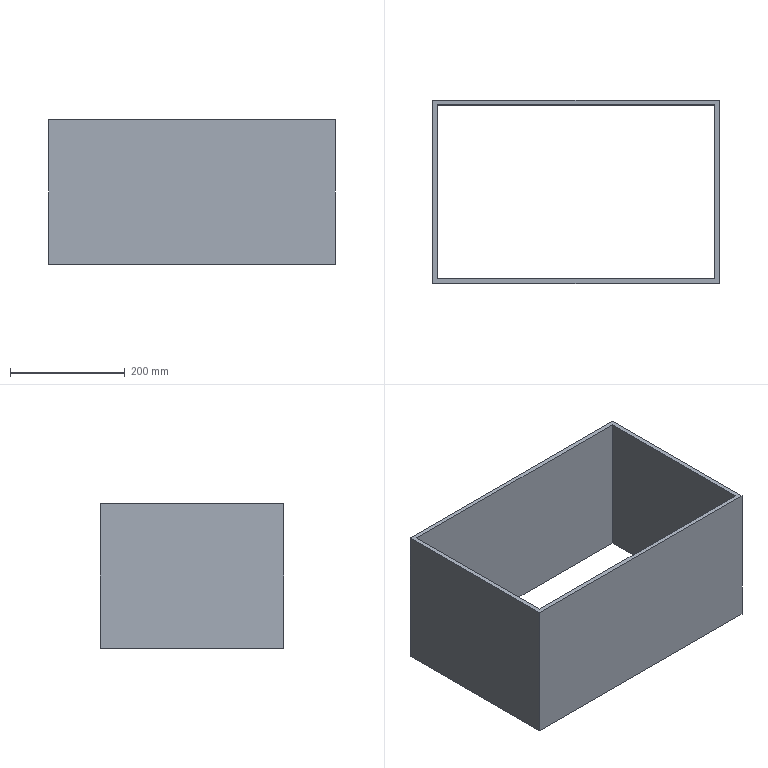Part | SolidWorks | features Extrusion 1 | 1 solid | 10 faces | box 500 x 320 x 252.7 mm | volume 3250733 mm3 | plane 10
STEP:
#1=CARTESIAN_POINT('',(0.,320.,252.7));
#2=VERTEX_POINT('',#1);
#3=CARTESIAN_POINT('',(0.,0.,252.7));
#4=VERTEX_POINT('',#3);
#5=CARTESIAN_POINT('',(0.,0.,252.7));
#6=DIRECTION('',(0.,-1.,0.));
#7=VECTOR('',#6,1000.);
#8=LINE('',#5,#7);
#9=EDGE_CURVE('',#2,#4,#8,.T.);
#10=ORIENTED_EDGE('',*,*,#9,.T.);
#11=CARTESIAN_POINT('',(500.,0.,252.7));
#12=VERTEX_POINT('',#11);
#13=CARTESIAN_POINT('',(0.,0.,252.7));
#14=DIRECTION('',(1.,0.,0.));
#15=VECTOR('',#14,1000.);
#16=LINE('',#13,#15);
#17=EDGE_CURVE('',#4,#12,#16,.T.);
#18=ORIENTED_EDGE('',*,*,#17,.T.);
#19=CARTESIAN_POINT('',(500.,320.,252.7));
#20=VERTEX_POINT('',#19);
#21=CARTESIAN_POINT('',(500.,0.,252.7));
#22=DIRECTION('',(0.,1.,0.));
#23=VECTOR('',#22,1000.);
#24=LINE('',#21,#23);
#25=EDGE_CURVE('',#12,#20,#24,.T.);
#26=ORIENTED_EDGE('',*,*,#25,.T.);
#27=CARTESIAN_POINT('',(0.,320.,252.7));
#28=DIRECTION('',(-1.,0.,0.));
#29=VECTOR('',#28,1000.);
#30=LINE('',#27,#29);
#31=EDGE_CURVE('',#20,#2,#30,.T.);
#32=ORIENTED_EDGE('',*,*,#31,.T.);
#33=EDGE_LOOP('',(#10,#18,#26,#32));
#34=FACE_OUTER_BOUND('',#33,.T.);
#35=CARTESIAN_POINT('',(8.,312.,252.7));
#36=VERTEX_POINT('',#35);
#37=CARTESIAN_POINT('',(8.,8.,252.7));
#38=VERTEX_POINT('',#37);
#39=CARTESIAN_POINT('',(8.,312.,252.7));
#40=DIRECTION('',(0.,-1.,0.));
#41=VECTOR('',#40,1000.);
#42=LINE('',#39,#41);
#43=EDGE_CURVE('',#36,#38,#42,.T.);
#44=ORIENTED_EDGE('',*,*,#43,.F.);
#45=CARTESIAN_POINT('',(492.,312.,252.7));
#46=VERTEX_POINT('',#45);
#47=CARTESIAN_POINT('',(8.,312.,252.7));
#48=DIRECTION('',(-1.,0.,0.));
#49=VECTOR('',#48,1000.);
#50=LINE('',#47,#49);
#51=EDGE_CURVE('',#46,#36,#50,.T.);
#52=ORIENTED_EDGE('',*,*,#51,.F.);
#53=CARTESIAN_POINT('',(492.,8.,252.7));
#54=VERTEX_POINT('',#53);
#55=CARTESIAN_POINT('',(492.,312.,252.7));
#56=DIRECTION('',(0.,1.,0.));
#57=VECTOR('',#56,1000.);
#58=LINE('',#55,#57);
#59=EDGE_CURVE('',#54,#46,#58,.T.);
#60=ORIENTED_EDGE('',*,*,#59,.F.);
#61=CARTESIAN_POINT('',(8.,8.,252.7));
#62=DIRECTION('',(1.,0.,0.));
#63=VECTOR('',#62,1000.);
#64=LINE('',#61,#63);
#65=EDGE_CURVE('',#38,#54,#64,.T.);
#66=ORIENTED_EDGE('',*,*,#65,.F.);
#67=EDGE_LOOP('',(#44,#52,#60,#66));
#68=FACE_BOUND('',#67,.T.);
#69=CARTESIAN_POINT('',(0.,0.,252.7));
#70=DIRECTION('',(0.,0.,-1.));
#71=DIRECTION('',(-1.,0.,0.));
#72=AXIS2_PLACEMENT_3D('',#69,#70,#71);
#73=PLANE('',#72);
#74=ADVANCED_FACE('',(#34,#68),#73,.F.);
#75=CARTESIAN_POINT('',(0.,320.,0.));
#76=VERTEX_POINT('',#75);
#77=CARTESIAN_POINT('',(0.,0.,0.));
#78=VERTEX_POINT('',#77);
#79=CARTESIAN_POINT('',(0.,0.,0.));
#80=DIRECTION('',(0.,-1.,0.));
#81=VECTOR('',#80,1000.);
#82=LINE('',#79,#81);
#83=EDGE_CURVE('',#76,#78,#82,.T.);
#84=ORIENTED_EDGE('',*,*,#83,.F.);
#85=CARTESIAN_POINT('',(500.,320.,0.));
#86=VERTEX_POINT('',#85);
#87=CARTESIAN_POINT('',(0.,320.,0.));
#88=DIRECTION('',(-1.,0.,0.));
#89=VECTOR('',#88,1000.);
#90=LINE('',#87,#89);
#91=EDGE_CURVE('',#86,#76,#90,.T.);
#92=ORIENTED_EDGE('',*,*,#91,.F.);
#93=CARTESIAN_POINT('',(500.,0.,0.));
#94=VERTEX_POINT('',#93);
#95=CARTESIAN_POINT('',(500.,0.,0.));
#96=DIRECTION('',(0.,1.,0.));
#97=VECTOR('',#96,1000.);
#98=LINE('',#95,#97);
#99=EDGE_CURVE('',#94,#86,#98,.T.);
#100=ORIENTED_EDGE('',*,*,#99,.F.);
#101=CARTESIAN_POINT('',(0.,0.,0.));
#102=DIRECTION('',(1.,0.,0.));
#103=VECTOR('',#102,1000.);
#104=LINE('',#101,#103);
#105=EDGE_CURVE('',#78,#94,#104,.T.);
#106=ORIENTED_EDGE('',*,*,#105,.F.);
#107=EDGE_LOOP('',(#84,#92,#100,#106));
#108=FACE_OUTER_BOUND('',#107,.T.);
#109=CARTESIAN_POINT('',(492.,312.,0.));
#110=VERTEX_POINT('',#109);
#111=CARTESIAN_POINT('',(8.,312.,0.));
#112=VERTEX_POINT('',#111);
#113=CARTESIAN_POINT('',(8.,312.,0.));
#114=DIRECTION('',(-1.,0.,0.));
#115=VECTOR('',#114,1000.);
#116=LINE('',#113,#115);
#117=EDGE_CURVE('',#110,#112,#116,.T.);
#118=ORIENTED_EDGE('',*,*,#117,.T.);
#119=CARTESIAN_POINT('',(8.,8.,0.));
#120=VERTEX_POINT('',#119);
#121=CARTESIAN_POINT('',(8.,312.,0.));
#122=DIRECTION('',(0.,-1.,0.));
#123=VECTOR('',#122,1000.);
#124=LINE('',#121,#123);
#125=EDGE_CURVE('',#112,#120,#124,.T.);
#126=ORIENTED_EDGE('',*,*,#125,.T.);
#127=CARTESIAN_POINT('',(492.,8.,0.));
#128=VERTEX_POINT('',#127);
#129=CARTESIAN_POINT('',(8.,8.,0.));
#130=DIRECTION('',(1.,0.,0.));
#131=VECTOR('',#130,1000.);
#132=LINE('',#129,#131);
#133=EDGE_CURVE('',#120,#128,#132,.T.);
#134=ORIENTED_EDGE('',*,*,#133,.T.);
#135=CARTESIAN_POINT('',(492.,312.,0.));
#136=DIRECTION('',(0.,1.,0.));
#137=VECTOR('',#136,1000.);
#138=LINE('',#135,#137);
#139=EDGE_CURVE('',#128,#110,#138,.T.);
#140=ORIENTED_EDGE('',*,*,#139,.T.);
#141=EDGE_LOOP('',(#118,#126,#134,#140));
#142=FACE_BOUND('',#141,.T.);
#143=CARTESIAN_POINT('',(0.,0.,0.));
#144=DIRECTION('',(0.,0.,-1.));
#145=DIRECTION('',(-1.,0.,0.));
#146=AXIS2_PLACEMENT_3D('',#143,#144,#145);
#147=PLANE('',#146);
#148=ADVANCED_FACE('',(#108,#142),#147,.T.);
#149=ORIENTED_EDGE('',*,*,#83,.T.);
#150=CARTESIAN_POINT('',(0.,0.,252.7));
#151=DIRECTION('',(0.,0.,-1.));
#152=VECTOR('',#151,1000.);
#153=LINE('',#150,#152);
#154=EDGE_CURVE('',#4,#78,#153,.T.);
#155=ORIENTED_EDGE('',*,*,#154,.F.);
#156=ORIENTED_EDGE('',*,*,#9,.F.);
#157=CARTESIAN_POINT('',(0.,320.,252.7));
#158=DIRECTION('',(0.,0.,-1.));
#159=VECTOR('',#158,1000.);
#160=LINE('',#157,#159);
#161=EDGE_CURVE('',#2,#76,#160,.T.);
#162=ORIENTED_EDGE('',*,*,#161,.T.);
#163=EDGE_LOOP('',(#149,#155,#156,#162));
#164=FACE_OUTER_BOUND('',#163,.T.);
#165=CARTESIAN_POINT('',(0.,0.,252.7));
#166=DIRECTION('',(1.,0.,0.));
#167=DIRECTION('',(0.,0.,-1.));
#168=AXIS2_PLACEMENT_3D('',#165,#166,#167);
#169=PLANE('',#168);
#170=ADVANCED_FACE('',(#164),#169,.F.);
#171=ORIENTED_EDGE('',*,*,#105,.T.);
#172=CARTESIAN_POINT('',(500.,0.,252.7));
#173=DIRECTION('',(0.,0.,-1.));
#174=VECTOR('',#173,1000.);
#175=LINE('',#172,#174);
#176=EDGE_CURVE('',#12,#94,#175,.T.);
#177=ORIENTED_EDGE('',*,*,#176,.F.);
#178=ORIENTED_EDGE('',*,*,#17,.F.);
#179=ORIENTED_EDGE('',*,*,#154,.T.);
#180=EDGE_LOOP('',(#171,#177,#178,#179));
#181=FACE_OUTER_BOUND('',#180,.T.);
#182=CARTESIAN_POINT('',(0.,0.,252.7));
#183=DIRECTION('',(0.,1.,0.));
#184=DIRECTION('',(0.,0.,1.));
#185=AXIS2_PLACEMENT_3D('',#182,#183,#184);
#186=PLANE('',#185);
#187=ADVANCED_FACE('',(#181),#186,.F.);
#188=ORIENTED_EDGE('',*,*,#99,.T.);
#189=CARTESIAN_POINT('',(500.,320.,252.7));
#190=DIRECTION('',(0.,0.,-1.));
#191=VECTOR('',#190,1000.);
#192=LINE('',#189,#191);
#193=EDGE_CURVE('',#20,#86,#192,.T.);
#194=ORIENTED_EDGE('',*,*,#193,.F.);
#195=ORIENTED_EDGE('',*,*,#25,.F.);
#196=ORIENTED_EDGE('',*,*,#176,.T.);
#197=EDGE_LOOP('',(#188,#194,#195,#196));
#198=FACE_OUTER_BOUND('',#197,.T.);
#199=CARTESIAN_POINT('',(500.,0.,252.7));
#200=DIRECTION('',(-1.,0.,0.));
#201=DIRECTION('',(0.,0.,1.));
#202=AXIS2_PLACEMENT_3D('',#199,#200,#201);
#203=PLANE('',#202);
#204=ADVANCED_FACE('',(#198),#203,.F.);
#205=ORIENTED_EDGE('',*,*,#91,.T.);
#206=ORIENTED_EDGE('',*,*,#161,.F.);
#207=ORIENTED_EDGE('',*,*,#31,.F.);
#208=ORIENTED_EDGE('',*,*,#193,.T.);
#209=EDGE_LOOP('',(#205,#206,#207,#208));
#210=FACE_OUTER_BOUND('',#209,.T.);
#211=CARTESIAN_POINT('',(0.,320.,252.7));
#212=DIRECTION('',(0.,-1.,0.));
#213=DIRECTION('',(0.,0.,-1.));
#214=AXIS2_PLACEMENT_3D('',#211,#212,#213);
#215=PLANE('',#214);
#216=ADVANCED_FACE('',(#210),#215,.F.);
#217=ORIENTED_EDGE('',*,*,#125,.F.);
#218=CARTESIAN_POINT('',(8.,312.,252.7));
#219=DIRECTION('',(0.,0.,-1.));
#220=VECTOR('',#219,1000.);
#221=LINE('',#218,#220);
#222=EDGE_CURVE('',#36,#112,#221,.T.);
#223=ORIENTED_EDGE('',*,*,#222,.F.);
#224=ORIENTED_EDGE('',*,*,#43,.T.);
#225=CARTESIAN_POINT('',(8.,8.,252.7));
#226=DIRECTION('',(0.,0.,-1.));
#227=VECTOR('',#226,1000.);
#228=LINE('',#225,#227);
#229=EDGE_CURVE('',#38,#120,#228,.T.);
#230=ORIENTED_EDGE('',*,*,#229,.T.);
#231=EDGE_LOOP('',(#217,#223,#224,#230));
#232=FACE_OUTER_BOUND('',#231,.T.);
#233=CARTESIAN_POINT('',(8.,312.,252.7));
#234=DIRECTION('',(1.,0.,0.));
#235=DIRECTION('',(0.,1.,0.));
#236=AXIS2_PLACEMENT_3D('',#233,#234,#235);
#237=PLANE('',#236);
#238=ADVANCED_FACE('',(#232),#237,.T.);
#239=ORIENTED_EDGE('',*,*,#133,.F.);
#240=ORIENTED_EDGE('',*,*,#229,.F.);
#241=ORIENTED_EDGE('',*,*,#65,.T.);
#242=CARTESIAN_POINT('',(492.,8.,252.7));
#243=DIRECTION('',(0.,0.,-1.));
#244=VECTOR('',#243,1000.);
#245=LINE('',#242,#244);
#246=EDGE_CURVE('',#54,#128,#245,.T.);
#247=ORIENTED_EDGE('',*,*,#246,.T.);
#248=EDGE_LOOP('',(#239,#240,#241,#247));
#249=FACE_OUTER_BOUND('',#248,.T.);
#250=CARTESIAN_POINT('',(8.,8.,252.7));
#251=DIRECTION('',(0.,1.,0.));
#252=DIRECTION('',(-1.,0.,0.));
#253=AXIS2_PLACEMENT_3D('',#250,#251,#252);
#254=PLANE('',#253);
#255=ADVANCED_FACE('',(#249),#254,.T.);
#256=ORIENTED_EDGE('',*,*,#139,.F.);
#257=ORIENTED_EDGE('',*,*,#246,.F.);
#258=ORIENTED_EDGE('',*,*,#59,.T.);
#259=CARTESIAN_POINT('',(492.,312.,252.7));
#260=DIRECTION('',(0.,0.,-1.));
#261=VECTOR('',#260,1000.);
#262=LINE('',#259,#261);
#263=EDGE_CURVE('',#46,#110,#262,.T.);
#264=ORIENTED_EDGE('',*,*,#263,.T.);
#265=EDGE_LOOP('',(#256,#257,#258,#264));
#266=FACE_OUTER_BOUND('',#265,.T.);
#267=CARTESIAN_POINT('',(492.,312.,252.7));
#268=DIRECTION('',(-1.,0.,0.));
#269=DIRECTION('',(0.,-1.,0.));
#270=AXIS2_PLACEMENT_3D('',#267,#268,#269);
#271=PLANE('',#270);
#272=ADVANCED_FACE('',(#266),#271,.T.);
#273=ORIENTED_EDGE('',*,*,#117,.F.);
#274=ORIENTED_EDGE('',*,*,#263,.F.);
#275=ORIENTED_EDGE('',*,*,#51,.T.);
#276=ORIENTED_EDGE('',*,*,#222,.T.);
#277=EDGE_LOOP('',(#273,#274,#275,#276));
#278=FACE_OUTER_BOUND('',#277,.T.);
#279=CARTESIAN_POINT('',(8.,312.,252.7));
#280=DIRECTION('',(0.,-1.,0.));
#281=DIRECTION('',(0.,0.,-1.));
#282=AXIS2_PLACEMENT_3D('',#279,#280,#281);
#283=PLANE('',#282);
#284=ADVANCED_FACE('',(#278),#283,.T.);
#285=CLOSED_SHELL('',(#74,#148,#170,#187,#204,#216,#238,#255,#272,#284));
#286=MANIFOLD_SOLID_BREP('',#285);
#287=CARTESIAN_POINT('',(0.,0.,0.));
#288=DIRECTION('',(0.,0.,1.));
#289=DIRECTION('',(1.,0.,0.));
#290=AXIS2_PLACEMENT_3D('',#287,#288,#289);
#291=(LENGTH_UNIT()NAMED_UNIT(*)SI_UNIT(.MILLI.,.METRE.));
#292=UNCERTAINTY_MEASURE_WITH_UNIT(LENGTH_MEASURE(0.00001),#291,'','');
#293=(NAMED_UNIT(*)PLANE_ANGLE_UNIT()SI_UNIT($,.RADIAN.));
#294=(NAMED_UNIT(*)SI_UNIT($,.STERADIAN.)SOLID_ANGLE_UNIT());
#295=(GEOMETRIC_REPRESENTATION_CONTEXT(3)GLOBAL_UNCERTAINTY_ASSIGNED_CONTEXT((#292))GLOBAL_UNIT_ASSIGNED_CONTEXT((#291,#293,#294))REPRESENTATION_CONTEXT('',''));
#296=ADVANCED_BREP_SHAPE_REPRESENTATION('',(#286,#290),#295);